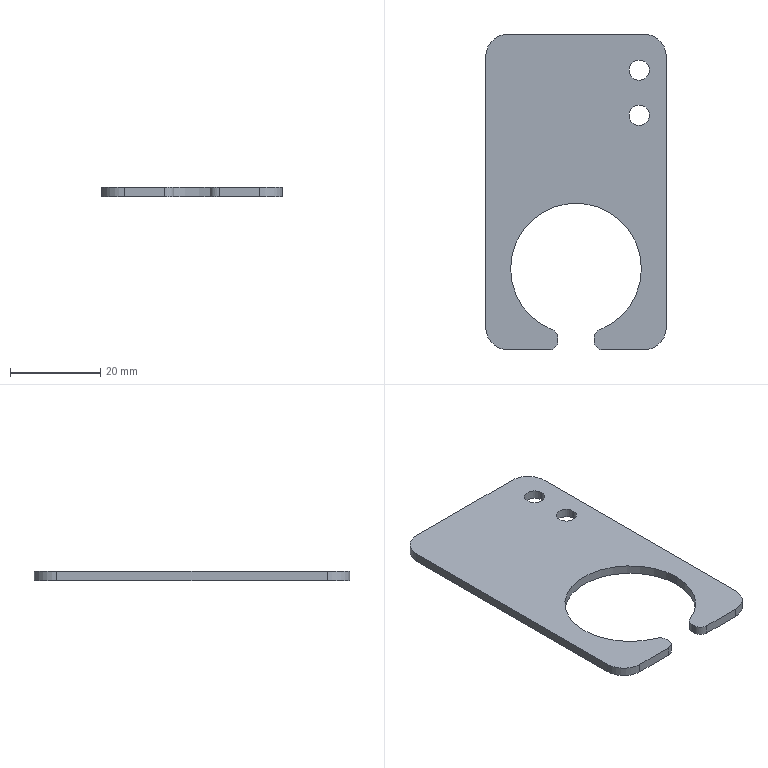Part | STEP file | 02-04 corrugated tube mounting seat (Default) | 1 solid | 24 faces | box 40 x 70 x 2 mm | volume 4109 mm3 | cylinder 15 | plane 9 | commonest cylinder face diameters 4 x4 4.5 x4 10 x4 29 x3
STEP:
#1=CARTESIAN_POINT('',(11.75,17.,-2.));
#2=VERTEX_POINT('',#1);
#3=CARTESIAN_POINT('',(16.25,17.,-2.));
#4=VERTEX_POINT('',#3);
#5=CARTESIAN_POINT('',(14.,17.,-2.));
#6=DIRECTION('',(0.,0.,1.));
#7=DIRECTION('',(1.,0.,0.));
#8=AXIS2_PLACEMENT_3D('',#5,#6,#7);
#9=CIRCLE('',#8,2.25);
#10=EDGE_CURVE('',#2,#4,#9,.T.);
#11=ORIENTED_EDGE('',*,*,#10,.F.);
#12=CARTESIAN_POINT('',(11.75,17.,0.));
#13=VERTEX_POINT('',#12);
#14=CARTESIAN_POINT('',(11.75,17.,-10.));
#15=DIRECTION('',(0.,0.,1.));
#16=VECTOR('',#15,1000.);
#17=LINE('',#14,#16);
#18=EDGE_CURVE('',#2,#13,#17,.T.);
#19=ORIENTED_EDGE('',*,*,#18,.T.);
#20=CARTESIAN_POINT('',(16.25,17.,0.));
#21=VERTEX_POINT('',#20);
#22=CARTESIAN_POINT('',(14.,17.,0.));
#23=DIRECTION('',(0.,0.,1.));
#24=DIRECTION('',(1.,0.,0.));
#25=AXIS2_PLACEMENT_3D('',#22,#23,#24);
#26=CIRCLE('',#25,2.25);
#27=EDGE_CURVE('',#13,#21,#26,.T.);
#28=ORIENTED_EDGE('',*,*,#27,.T.);
#29=CARTESIAN_POINT('',(16.25,17.,-10.));
#30=DIRECTION('',(0.,0.,1.));
#31=VECTOR('',#30,1000.);
#32=LINE('',#29,#31);
#33=EDGE_CURVE('',#4,#21,#32,.T.);
#34=ORIENTED_EDGE('',*,*,#33,.F.);
#35=EDGE_LOOP('',(#11,#19,#28,#34));
#36=FACE_OUTER_BOUND('',#35,.T.);
#37=CARTESIAN_POINT('',(14.,17.,-10.));
#38=DIRECTION('',(0.,0.,1.));
#39=DIRECTION('',(1.,0.,0.));
#40=AXIS2_PLACEMENT_3D('',#37,#38,#39);
#41=CYLINDRICAL_SURFACE('',#40,2.25);
#42=ADVANCED_FACE('',(#36),#41,.F.);
#43=CARTESIAN_POINT('',(11.75,27.,-2.));
#44=VERTEX_POINT('',#43);
#45=CARTESIAN_POINT('',(16.25,27.,-2.));
#46=VERTEX_POINT('',#45);
#47=CARTESIAN_POINT('',(14.,27.,-2.));
#48=DIRECTION('',(0.,0.,1.));
#49=DIRECTION('',(1.,0.,0.));
#50=AXIS2_PLACEMENT_3D('',#47,#48,#49);
#51=CIRCLE('',#50,2.25);
#52=EDGE_CURVE('',#44,#46,#51,.T.);
#53=ORIENTED_EDGE('',*,*,#52,.F.);
#54=CARTESIAN_POINT('',(11.75,27.,0.));
#55=VERTEX_POINT('',#54);
#56=CARTESIAN_POINT('',(11.75,27.,-10.));
#57=DIRECTION('',(0.,0.,1.));
#58=VECTOR('',#57,1000.);
#59=LINE('',#56,#58);
#60=EDGE_CURVE('',#44,#55,#59,.T.);
#61=ORIENTED_EDGE('',*,*,#60,.T.);
#62=CARTESIAN_POINT('',(16.25,27.,0.));
#63=VERTEX_POINT('',#62);
#64=CARTESIAN_POINT('',(14.,27.,0.));
#65=DIRECTION('',(0.,0.,1.));
#66=DIRECTION('',(1.,0.,0.));
#67=AXIS2_PLACEMENT_3D('',#64,#65,#66);
#68=CIRCLE('',#67,2.25);
#69=EDGE_CURVE('',#55,#63,#68,.T.);
#70=ORIENTED_EDGE('',*,*,#69,.T.);
#71=CARTESIAN_POINT('',(16.25,27.,-10.));
#72=DIRECTION('',(0.,0.,1.));
#73=VECTOR('',#72,1000.);
#74=LINE('',#71,#73);
#75=EDGE_CURVE('',#46,#63,#74,.T.);
#76=ORIENTED_EDGE('',*,*,#75,.F.);
#77=EDGE_LOOP('',(#53,#61,#70,#76));
#78=FACE_OUTER_BOUND('',#77,.T.);
#79=CARTESIAN_POINT('',(14.,27.,-10.));
#80=DIRECTION('',(0.,0.,1.));
#81=DIRECTION('',(1.,0.,0.));
#82=AXIS2_PLACEMENT_3D('',#79,#80,#81);
#83=CYLINDRICAL_SURFACE('',#82,2.25);
#84=ADVANCED_FACE('',(#78),#83,.F.);
#85=CARTESIAN_POINT('',(-14.5,-17.,-2.));
#86=VERTEX_POINT('',#85);
#87=CARTESIAN_POINT('',(-5.273,-30.507,-2.));
#88=VERTEX_POINT('',#87);
#89=CARTESIAN_POINT('',(0.,-17.,-2.));
#90=DIRECTION('',(0.,0.,1.));
#91=DIRECTION('',(1.,0.,0.));
#92=AXIS2_PLACEMENT_3D('',#89,#90,#91);
#93=CIRCLE('',#92,14.5);
#94=EDGE_CURVE('',#86,#88,#93,.T.);
#95=ORIENTED_EDGE('',*,*,#94,.F.);
#96=CARTESIAN_POINT('',(-14.5,-17.,0.));
#97=VERTEX_POINT('',#96);
#98=CARTESIAN_POINT('',(-14.5,-17.,-10.));
#99=DIRECTION('',(0.,0.,1.));
#100=VECTOR('',#99,1000.);
#101=LINE('',#98,#100);
#102=EDGE_CURVE('',#86,#97,#101,.T.);
#103=ORIENTED_EDGE('',*,*,#102,.T.);
#104=CARTESIAN_POINT('',(-5.273,-30.507,0.));
#105=VERTEX_POINT('',#104);
#106=CARTESIAN_POINT('',(0.,-17.,0.));
#107=DIRECTION('',(0.,0.,1.));
#108=DIRECTION('',(1.,0.,0.));
#109=AXIS2_PLACEMENT_3D('',#106,#107,#108);
#110=CIRCLE('',#109,14.5);
#111=EDGE_CURVE('',#97,#105,#110,.T.);
#112=ORIENTED_EDGE('',*,*,#111,.T.);
#113=CARTESIAN_POINT('',(-5.273,-30.507,-10.));
#114=DIRECTION('',(0.,0.,-1.));
#115=VECTOR('',#114,1000.);
#116=LINE('',#113,#115);
#117=EDGE_CURVE('',#105,#88,#116,.T.);
#118=ORIENTED_EDGE('',*,*,#117,.T.);
#119=EDGE_LOOP('',(#95,#103,#112,#118));
#120=FACE_OUTER_BOUND('',#119,.T.);
#121=CARTESIAN_POINT('',(0.,-17.,-10.));
#122=DIRECTION('',(0.,0.,1.));
#123=DIRECTION('',(1.,0.,0.));
#124=AXIS2_PLACEMENT_3D('',#121,#122,#123);
#125=CYLINDRICAL_SURFACE('',#124,14.5);
#126=ADVANCED_FACE('',(#120),#125,.F.);
#127=ORIENTED_EDGE('',*,*,#102,.F.);
#128=CARTESIAN_POINT('',(14.5,-17.,-2.));
#129=VERTEX_POINT('',#128);
#130=CARTESIAN_POINT('',(0.,-17.,-2.));
#131=DIRECTION('',(0.,0.,1.));
#132=DIRECTION('',(1.,0.,0.));
#133=AXIS2_PLACEMENT_3D('',#130,#131,#132);
#134=CIRCLE('',#133,14.5);
#135=EDGE_CURVE('',#129,#86,#134,.T.);
#136=ORIENTED_EDGE('',*,*,#135,.F.);
#137=CARTESIAN_POINT('',(14.5,-17.,0.));
#138=VERTEX_POINT('',#137);
#139=CARTESIAN_POINT('',(14.5,-17.,-10.));
#140=DIRECTION('',(0.,0.,1.));
#141=VECTOR('',#140,1000.);
#142=LINE('',#139,#141);
#143=EDGE_CURVE('',#129,#138,#142,.T.);
#144=ORIENTED_EDGE('',*,*,#143,.T.);
#145=CARTESIAN_POINT('',(0.,-17.,0.));
#146=DIRECTION('',(0.,0.,1.));
#147=DIRECTION('',(1.,0.,0.));
#148=AXIS2_PLACEMENT_3D('',#145,#146,#147);
#149=CIRCLE('',#148,14.5);
#150=EDGE_CURVE('',#138,#97,#149,.T.);
#151=ORIENTED_EDGE('',*,*,#150,.T.);
#152=EDGE_LOOP('',(#127,#136,#144,#151));
#153=FACE_OUTER_BOUND('',#152,.T.);
#154=CARTESIAN_POINT('',(0.,-17.,-10.));
#155=DIRECTION('',(0.,0.,1.));
#156=DIRECTION('',(1.,0.,0.));
#157=AXIS2_PLACEMENT_3D('',#154,#155,#156);
#158=CYLINDRICAL_SURFACE('',#157,14.5);
#159=ADVANCED_FACE('',(#153),#158,.F.);
#160=CARTESIAN_POINT('',(6.,-35.,-2.));
#161=VERTEX_POINT('',#160);
#162=CARTESIAN_POINT('',(15.,-35.,-2.));
#163=VERTEX_POINT('',#162);
#164=CARTESIAN_POINT('',(-20.,-35.,-2.));
#165=DIRECTION('',(1.,0.,0.));
#166=VECTOR('',#165,1000.);
#167=LINE('',#164,#166);
#168=EDGE_CURVE('',#161,#163,#167,.T.);
#169=ORIENTED_EDGE('',*,*,#168,.T.);
#170=CARTESIAN_POINT('',(15.,-35.,0.));
#171=VERTEX_POINT('',#170);
#172=CARTESIAN_POINT('',(15.,-35.,-2.));
#173=DIRECTION('',(0.,0.,1.));
#174=VECTOR('',#173,1000.);
#175=LINE('',#172,#174);
#176=EDGE_CURVE('',#163,#171,#175,.T.);
#177=ORIENTED_EDGE('',*,*,#176,.T.);
#178=CARTESIAN_POINT('',(6.,-35.,0.));
#179=VERTEX_POINT('',#178);
#180=CARTESIAN_POINT('',(-20.,-35.,0.));
#181=DIRECTION('',(1.,0.,0.));
#182=VECTOR('',#181,1000.);
#183=LINE('',#180,#182);
#184=EDGE_CURVE('',#179,#171,#183,.T.);
#185=ORIENTED_EDGE('',*,*,#184,.F.);
#186=CARTESIAN_POINT('',(6.,-35.,-2.));
#187=DIRECTION('',(0.,0.,-1.));
#188=VECTOR('',#187,1000.);
#189=LINE('',#186,#188);
#190=EDGE_CURVE('',#179,#161,#189,.T.);
#191=ORIENTED_EDGE('',*,*,#190,.T.);
#192=EDGE_LOOP('',(#169,#177,#185,#191));
#193=FACE_OUTER_BOUND('',#192,.T.);
#194=CARTESIAN_POINT('',(-20.,-35.,-2.));
#195=DIRECTION('',(0.,-1.,0.));
#196=DIRECTION('',(0.,0.,-1.));
#197=AXIS2_PLACEMENT_3D('',#194,#195,#196);
#198=PLANE('',#197);
#199=ADVANCED_FACE('',(#193),#198,.T.);
#200=CARTESIAN_POINT('',(20.,-30.,-2.));
#201=VERTEX_POINT('',#200);
#202=CARTESIAN_POINT('',(20.,30.,-2.));
#203=VERTEX_POINT('',#202);
#204=CARTESIAN_POINT('',(20.,35.,-2.));
#205=DIRECTION('',(0.,1.,0.));
#206=VECTOR('',#205,1000.);
#207=LINE('',#204,#206);
#208=EDGE_CURVE('',#201,#203,#207,.T.);
#209=ORIENTED_EDGE('',*,*,#208,.T.);
#210=CARTESIAN_POINT('',(20.,30.,0.));
#211=VERTEX_POINT('',#210);
#212=CARTESIAN_POINT('',(20.,30.,-2.));
#213=DIRECTION('',(0.,0.,1.));
#214=VECTOR('',#213,1000.);
#215=LINE('',#212,#214);
#216=EDGE_CURVE('',#203,#211,#215,.T.);
#217=ORIENTED_EDGE('',*,*,#216,.T.);
#218=CARTESIAN_POINT('',(20.,-30.,0.));
#219=VERTEX_POINT('',#218);
#220=CARTESIAN_POINT('',(20.,35.,0.));
#221=DIRECTION('',(0.,1.,0.));
#222=VECTOR('',#221,1000.);
#223=LINE('',#220,#222);
#224=EDGE_CURVE('',#219,#211,#223,.T.);
#225=ORIENTED_EDGE('',*,*,#224,.F.);
#226=CARTESIAN_POINT('',(20.,-30.,-2.));
#227=DIRECTION('',(0.,0.,-1.));
#228=VECTOR('',#227,1000.);
#229=LINE('',#226,#228);
#230=EDGE_CURVE('',#219,#201,#229,.T.);
#231=ORIENTED_EDGE('',*,*,#230,.T.);
#232=EDGE_LOOP('',(#209,#217,#225,#231));
#233=FACE_OUTER_BOUND('',#232,.T.);
#234=CARTESIAN_POINT('',(20.,35.,-2.));
#235=DIRECTION('',(1.,0.,0.));
#236=DIRECTION('',(0.,1.,0.));
#237=AXIS2_PLACEMENT_3D('',#234,#235,#236);
#238=PLANE('',#237);
#239=ADVANCED_FACE('',(#233),#238,.T.);
#240=CARTESIAN_POINT('',(-15.,-35.,0.));
#241=VERTEX_POINT('',#240);
#242=CARTESIAN_POINT('',(-6.,-35.,0.));
#243=VERTEX_POINT('',#242);
#244=CARTESIAN_POINT('',(-20.,-35.,0.));
#245=DIRECTION('',(1.,0.,0.));
#246=VECTOR('',#245,1000.);
#247=LINE('',#244,#246);
#248=EDGE_CURVE('',#241,#243,#247,.T.);
#249=ORIENTED_EDGE('',*,*,#248,.F.);
#250=CARTESIAN_POINT('',(-15.,-35.,-2.));
#251=VERTEX_POINT('',#250);
#252=CARTESIAN_POINT('',(-15.,-35.,-2.));
#253=DIRECTION('',(0.,0.,-1.));
#254=VECTOR('',#253,1000.);
#255=LINE('',#252,#254);
#256=EDGE_CURVE('',#241,#251,#255,.T.);
#257=ORIENTED_EDGE('',*,*,#256,.T.);
#258=CARTESIAN_POINT('',(-6.,-35.,-2.));
#259=VERTEX_POINT('',#258);
#260=CARTESIAN_POINT('',(-20.,-35.,-2.));
#261=DIRECTION('',(1.,0.,0.));
#262=VECTOR('',#261,1000.);
#263=LINE('',#260,#262);
#264=EDGE_CURVE('',#251,#259,#263,.T.);
#265=ORIENTED_EDGE('',*,*,#264,.T.);
#266=CARTESIAN_POINT('',(-6.,-35.,0.));
#267=DIRECTION('',(0.,0.,1.));
#268=VECTOR('',#267,1000.);
#269=LINE('',#266,#268);
#270=EDGE_CURVE('',#259,#243,#269,.T.);
#271=ORIENTED_EDGE('',*,*,#270,.T.);
#272=EDGE_LOOP('',(#249,#257,#265,#271));
#273=FACE_OUTER_BOUND('',#272,.T.);
#274=CARTESIAN_POINT('',(-20.,-35.,-2.));
#275=DIRECTION('',(0.,-1.,0.));
#276=DIRECTION('',(0.,0.,-1.));
#277=AXIS2_PLACEMENT_3D('',#274,#275,#276);
#278=PLANE('',#277);
#279=ADVANCED_FACE('',(#273),#278,.T.);
#280=CARTESIAN_POINT('',(-20.,30.,0.));
#281=VERTEX_POINT('',#280);
#282=CARTESIAN_POINT('',(-20.,-30.,0.));
#283=VERTEX_POINT('',#282);
#284=CARTESIAN_POINT('',(-20.,35.,0.));
#285=DIRECTION('',(0.,-1.,0.));
#286=VECTOR('',#285,1000.);
#287=LINE('',#284,#286);
#288=EDGE_CURVE('',#281,#283,#287,.T.);
#289=ORIENTED_EDGE('',*,*,#288,.F.);
#290=CARTESIAN_POINT('',(-20.,30.,-2.));
#291=VERTEX_POINT('',#290);
#292=CARTESIAN_POINT('',(-20.,30.,-2.));
#293=DIRECTION('',(0.,0.,-1.));
#294=VECTOR('',#293,1000.);
#295=LINE('',#292,#294);
#296=EDGE_CURVE('',#281,#291,#295,.T.);
#297=ORIENTED_EDGE('',*,*,#296,.T.);
#298=CARTESIAN_POINT('',(-20.,-30.,-2.));
#299=VERTEX_POINT('',#298);
#300=CARTESIAN_POINT('',(-20.,35.,-2.));
#301=DIRECTION('',(0.,-1.,0.));
#302=VECTOR('',#301,1000.);
#303=LINE('',#300,#302);
#304=EDGE_CURVE('',#291,#299,#303,.T.);
#305=ORIENTED_EDGE('',*,*,#304,.T.);
#306=CARTESIAN_POINT('',(-20.,-30.,-2.));
#307=DIRECTION('',(0.,0.,1.));
#308=VECTOR('',#307,1000.);
#309=LINE('',#306,#308);
#310=EDGE_CURVE('',#299,#283,#309,.T.);
#311=ORIENTED_EDGE('',*,*,#310,.T.);
#312=EDGE_LOOP('',(#289,#297,#305,#311));
#313=FACE_OUTER_BOUND('',#312,.T.);
#314=CARTESIAN_POINT('',(-20.,35.,-2.));
#315=DIRECTION('',(-1.,0.,0.));
#316=DIRECTION('',(0.,-1.,0.));
#317=AXIS2_PLACEMENT_3D('',#314,#315,#316);
#318=PLANE('',#317);
#319=ADVANCED_FACE('',(#313),#318,.T.);
#320=CARTESIAN_POINT('',(15.,35.,0.));
#321=VERTEX_POINT('',#320);
#322=CARTESIAN_POINT('',(-15.,35.,0.));
#323=VERTEX_POINT('',#322);
#324=CARTESIAN_POINT('',(-20.,35.,0.));
#325=DIRECTION('',(-1.,0.,0.));
#326=VECTOR('',#325,1000.);
#327=LINE('',#324,#326);
#328=EDGE_CURVE('',#321,#323,#327,.T.);
#329=ORIENTED_EDGE('',*,*,#328,.F.);
#330=CARTESIAN_POINT('',(15.,35.,-2.));
#331=VERTEX_POINT('',#330);
#332=CARTESIAN_POINT('',(15.,35.,-2.));
#333=DIRECTION('',(0.,0.,-1.));
#334=VECTOR('',#333,1000.);
#335=LINE('',#332,#334);
#336=EDGE_CURVE('',#321,#331,#335,.T.);
#337=ORIENTED_EDGE('',*,*,#336,.T.);
#338=CARTESIAN_POINT('',(-15.,35.,-2.));
#339=VERTEX_POINT('',#338);
#340=CARTESIAN_POINT('',(-20.,35.,-2.));
#341=DIRECTION('',(-1.,0.,0.));
#342=VECTOR('',#341,1000.);
#343=LINE('',#340,#342);
#344=EDGE_CURVE('',#331,#339,#343,.T.);
#345=ORIENTED_EDGE('',*,*,#344,.T.);
#346=CARTESIAN_POINT('',(-15.,35.,-2.));
#347=DIRECTION('',(0.,0.,1.));
#348=VECTOR('',#347,1000.);
#349=LINE('',#346,#348);
#350=EDGE_CURVE('',#339,#323,#349,.T.);
#351=ORIENTED_EDGE('',*,*,#350,.T.);
#352=EDGE_LOOP('',(#329,#337,#345,#351));
#353=FACE_OUTER_BOUND('',#352,.T.);
#354=CARTESIAN_POINT('',(-20.,35.,-2.));
#355=DIRECTION('',(0.,1.,0.));
#356=DIRECTION('',(0.,0.,1.));
#357=AXIS2_PLACEMENT_3D('',#354,#355,#356);
#358=PLANE('',#357);
#359=ADVANCED_FACE('',(#353),#358,.T.);
#360=CARTESIAN_POINT('',(14.,17.,-2.));
#361=DIRECTION('',(0.,0.,1.));
#362=DIRECTION('',(1.,0.,0.));
#363=AXIS2_PLACEMENT_3D('',#360,#361,#362);
#364=CIRCLE('',#363,2.25);
#365=EDGE_CURVE('',#4,#2,#364,.T.);
#366=ORIENTED_EDGE('',*,*,#365,.T.);
#367=ORIENTED_EDGE('',*,*,#10,.T.);
#368=EDGE_LOOP('',(#366,#367));
#369=FACE_BOUND('',#368,.T.);
#370=CARTESIAN_POINT('',(14.,27.,-2.));
#371=DIRECTION('',(0.,0.,1.));
#372=DIRECTION('',(1.,0.,0.));
#373=AXIS2_PLACEMENT_3D('',#370,#371,#372);
#374=CIRCLE('',#373,2.25);
#375=EDGE_CURVE('',#46,#44,#374,.T.);
#376=ORIENTED_EDGE('',*,*,#375,.T.);
#377=ORIENTED_EDGE('',*,*,#52,.T.);
#378=EDGE_LOOP('',(#376,#377));
#379=FACE_BOUND('',#378,.T.);
#380=ORIENTED_EDGE('',*,*,#344,.F.);
#381=CARTESIAN_POINT('',(15.,30.,-2.));
#382=DIRECTION('',(0.,0.,-1.));
#383=DIRECTION('',(1.,0.,0.));
#384=AXIS2_PLACEMENT_3D('',#381,#382,#383);
#385=CIRCLE('',#384,5.);
#386=EDGE_CURVE('',#331,#203,#385,.T.);
#387=ORIENTED_EDGE('',*,*,#386,.T.);
#388=ORIENTED_EDGE('',*,*,#208,.F.);
#389=CARTESIAN_POINT('',(15.,-30.,-2.));
#390=DIRECTION('',(0.,0.,-1.));
#391=DIRECTION('',(1.,0.,0.));
#392=AXIS2_PLACEMENT_3D('',#389,#390,#391);
#393=CIRCLE('',#392,5.);
#394=EDGE_CURVE('',#201,#163,#393,.T.);
#395=ORIENTED_EDGE('',*,*,#394,.T.);
#396=ORIENTED_EDGE('',*,*,#168,.F.);
#397=CARTESIAN_POINT('',(4.,-33.,-2.));
#398=VERTEX_POINT('',#397);
#399=CARTESIAN_POINT('',(6.,-33.,-2.));
#400=DIRECTION('',(0.,0.,-1.));
#401=DIRECTION('',(1.,0.,0.));
#402=AXIS2_PLACEMENT_3D('',#399,#400,#401);
#403=CIRCLE('',#402,2.);
#404=EDGE_CURVE('',#161,#398,#403,.T.);
#405=ORIENTED_EDGE('',*,*,#404,.T.);
#406=CARTESIAN_POINT('',(4.,-32.37,-2.));
#407=VERTEX_POINT('',#406);
#408=CARTESIAN_POINT('',(4.,-35.,-2.));
#409=DIRECTION('',(0.,1.,0.));
#410=VECTOR('',#409,1000.);
#411=LINE('',#408,#410);
#412=EDGE_CURVE('',#398,#407,#411,.T.);
#413=ORIENTED_EDGE('',*,*,#412,.T.);
#414=CARTESIAN_POINT('',(5.273,-30.507,-2.));
#415=VERTEX_POINT('',#414);
#416=CARTESIAN_POINT('',(6.,-32.37,-2.));
#417=DIRECTION('',(0.,0.,-1.));
#418=DIRECTION('',(1.,0.,0.));
#419=AXIS2_PLACEMENT_3D('',#416,#417,#418);
#420=CIRCLE('',#419,2.);
#421=EDGE_CURVE('',#407,#415,#420,.T.);
#422=ORIENTED_EDGE('',*,*,#421,.T.);
#423=CARTESIAN_POINT('',(0.,-17.,-2.));
#424=DIRECTION('',(0.,0.,1.));
#425=DIRECTION('',(1.,0.,0.));
#426=AXIS2_PLACEMENT_3D('',#423,#424,#425);
#427=CIRCLE('',#426,14.5);
#428=EDGE_CURVE('',#415,#129,#427,.T.);
#429=ORIENTED_EDGE('',*,*,#428,.T.);
#430=ORIENTED_EDGE('',*,*,#135,.T.);
#431=ORIENTED_EDGE('',*,*,#94,.T.);
#432=CARTESIAN_POINT('',(-4.,-32.37,-2.));
#433=VERTEX_POINT('',#432);
#434=CARTESIAN_POINT('',(-6.,-32.37,-2.));
#435=DIRECTION('',(0.,0.,-1.));
#436=DIRECTION('',(1.,0.,0.));
#437=AXIS2_PLACEMENT_3D('',#434,#435,#436);
#438=CIRCLE('',#437,2.);
#439=EDGE_CURVE('',#88,#433,#438,.T.);
#440=ORIENTED_EDGE('',*,*,#439,.T.);
#441=CARTESIAN_POINT('',(-4.,-33.,-2.));
#442=VERTEX_POINT('',#441);
#443=CARTESIAN_POINT('',(-4.,-35.,-2.));
#444=DIRECTION('',(0.,-1.,0.));
#445=VECTOR('',#444,1000.);
#446=LINE('',#443,#445);
#447=EDGE_CURVE('',#433,#442,#446,.T.);
#448=ORIENTED_EDGE('',*,*,#447,.T.);
#449=CARTESIAN_POINT('',(-6.,-33.,-2.));
#450=DIRECTION('',(0.,0.,-1.));
#451=DIRECTION('',(1.,0.,0.));
#452=AXIS2_PLACEMENT_3D('',#449,#450,#451);
#453=CIRCLE('',#452,2.);
#454=EDGE_CURVE('',#442,#259,#453,.T.);
#455=ORIENTED_EDGE('',*,*,#454,.T.);
#456=ORIENTED_EDGE('',*,*,#264,.F.);
#457=CARTESIAN_POINT('',(-15.,-30.,-2.));
#458=DIRECTION('',(0.,0.,-1.));
#459=DIRECTION('',(1.,0.,0.));
#460=AXIS2_PLACEMENT_3D('',#457,#458,#459);
#461=CIRCLE('',#460,5.);
#462=EDGE_CURVE('',#251,#299,#461,.T.);
#463=ORIENTED_EDGE('',*,*,#462,.T.);
#464=ORIENTED_EDGE('',*,*,#304,.F.);
#465=CARTESIAN_POINT('',(-15.,30.,-2.));
#466=DIRECTION('',(0.,0.,-1.));
#467=DIRECTION('',(1.,0.,0.));
#468=AXIS2_PLACEMENT_3D('',#465,#466,#467);
#469=CIRCLE('',#468,5.);
#470=EDGE_CURVE('',#291,#339,#469,.T.);
#471=ORIENTED_EDGE('',*,*,#470,.T.);
#472=EDGE_LOOP('',(#380,#387,#388,#395,#396,#405,#413,#422,#429,#430,#431,#440,#448,#455,#456,#463,#464,#471));
#473=FACE_OUTER_BOUND('',#472,.T.);
#474=CARTESIAN_POINT('',(20.,-35.,-2.));
#475=DIRECTION('',(0.,0.,1.));
#476=DIRECTION('',(1.,0.,0.));
#477=AXIS2_PLACEMENT_3D('',#474,#475,#476);
#478=PLANE('',#477);
#479=ADVANCED_FACE('',(#369,#379,#473),#478,.F.);
#480=CARTESIAN_POINT('',(14.,17.,0.));
#481=DIRECTION('',(0.,0.,1.));
#482=DIRECTION('',(1.,0.,0.));
#483=AXIS2_PLACEMENT_3D('',#480,#481,#482);
#484=CIRCLE('',#483,2.25);
#485=EDGE_CURVE('',#21,#13,#484,.T.);
#486=ORIENTED_EDGE('',*,*,#485,.F.);
#487=ORIENTED_EDGE('',*,*,#27,.F.);
#488=EDGE_LOOP('',(#486,#487));
#489=FACE_BOUND('',#488,.T.);
#490=CARTESIAN_POINT('',(14.,27.,0.));
#491=DIRECTION('',(0.,0.,1.));
#492=DIRECTION('',(1.,0.,0.));
#493=AXIS2_PLACEMENT_3D('',#490,#491,#492);
#494=CIRCLE('',#493,2.25);
#495=EDGE_CURVE('',#63,#55,#494,.T.);
#496=ORIENTED_EDGE('',*,*,#495,.F.);
#497=ORIENTED_EDGE('',*,*,#69,.F.);
#498=EDGE_LOOP('',(#496,#497));
#499=FACE_BOUND('',#498,.T.);
#500=ORIENTED_EDGE('',*,*,#224,.T.);
#501=CARTESIAN_POINT('',(15.,30.,0.));
#502=DIRECTION('',(0.,0.,1.));
#503=DIRECTION('',(1.,0.,0.));
#504=AXIS2_PLACEMENT_3D('',#501,#502,#503);
#505=CIRCLE('',#504,5.);
#506=EDGE_CURVE('',#211,#321,#505,.T.);
#507=ORIENTED_EDGE('',*,*,#506,.T.);
#508=ORIENTED_EDGE('',*,*,#328,.T.);
#509=CARTESIAN_POINT('',(-15.,30.,0.));
#510=DIRECTION('',(0.,0.,1.));
#511=DIRECTION('',(1.,0.,0.));
#512=AXIS2_PLACEMENT_3D('',#509,#510,#511);
#513=CIRCLE('',#512,5.);
#514=EDGE_CURVE('',#323,#281,#513,.T.);
#515=ORIENTED_EDGE('',*,*,#514,.T.);
#516=ORIENTED_EDGE('',*,*,#288,.T.);
#517=CARTESIAN_POINT('',(-15.,-30.,0.));
#518=DIRECTION('',(0.,0.,1.));
#519=DIRECTION('',(1.,0.,0.));
#520=AXIS2_PLACEMENT_3D('',#517,#518,#519);
#521=CIRCLE('',#520,5.);
#522=EDGE_CURVE('',#283,#241,#521,.T.);
#523=ORIENTED_EDGE('',*,*,#522,.T.);
#524=ORIENTED_EDGE('',*,*,#248,.T.);
#525=CARTESIAN_POINT('',(-4.,-33.,0.));
#526=VERTEX_POINT('',#525);
#527=CARTESIAN_POINT('',(-6.,-33.,0.));
#528=DIRECTION('',(0.,0.,1.));
#529=DIRECTION('',(1.,0.,0.));
#530=AXIS2_PLACEMENT_3D('',#527,#528,#529);
#531=CIRCLE('',#530,2.);
#532=EDGE_CURVE('',#243,#526,#531,.T.);
#533=ORIENTED_EDGE('',*,*,#532,.T.);
#534=CARTESIAN_POINT('',(-4.,-32.37,0.));
#535=VERTEX_POINT('',#534);
#536=CARTESIAN_POINT('',(-4.,-30.937,0.));
#537=DIRECTION('',(0.,-1.,0.));
#538=VECTOR('',#537,1000.);
#539=LINE('',#536,#538);
#540=EDGE_CURVE('',#535,#526,#539,.T.);
#541=ORIENTED_EDGE('',*,*,#540,.F.);
#542=CARTESIAN_POINT('',(-6.,-32.37,0.));
#543=DIRECTION('',(0.,0.,1.));
#544=DIRECTION('',(1.,0.,0.));
#545=AXIS2_PLACEMENT_3D('',#542,#543,#544);
#546=CIRCLE('',#545,2.);
#547=EDGE_CURVE('',#535,#105,#546,.T.);
#548=ORIENTED_EDGE('',*,*,#547,.T.);
#549=ORIENTED_EDGE('',*,*,#111,.F.);
#550=ORIENTED_EDGE('',*,*,#150,.F.);
#551=CARTESIAN_POINT('',(5.273,-30.507,0.));
#552=VERTEX_POINT('',#551);
#553=CARTESIAN_POINT('',(0.,-17.,0.));
#554=DIRECTION('',(0.,0.,1.));
#555=DIRECTION('',(1.,0.,0.));
#556=AXIS2_PLACEMENT_3D('',#553,#554,#555);
#557=CIRCLE('',#556,14.5);
#558=EDGE_CURVE('',#552,#138,#557,.T.);
#559=ORIENTED_EDGE('',*,*,#558,.F.);
#560=CARTESIAN_POINT('',(4.,-32.37,0.));
#561=VERTEX_POINT('',#560);
#562=CARTESIAN_POINT('',(6.,-32.37,0.));
#563=DIRECTION('',(0.,0.,1.));
#564=DIRECTION('',(1.,0.,0.));
#565=AXIS2_PLACEMENT_3D('',#562,#563,#564);
#566=CIRCLE('',#565,2.);
#567=EDGE_CURVE('',#552,#561,#566,.T.);
#568=ORIENTED_EDGE('',*,*,#567,.T.);
#569=CARTESIAN_POINT('',(4.,-33.,0.));
#570=VERTEX_POINT('',#569);
#571=CARTESIAN_POINT('',(4.,-35.,0.));
#572=DIRECTION('',(0.,1.,0.));
#573=VECTOR('',#572,1000.);
#574=LINE('',#571,#573);
#575=EDGE_CURVE('',#570,#561,#574,.T.);
#576=ORIENTED_EDGE('',*,*,#575,.F.);
#577=CARTESIAN_POINT('',(6.,-33.,0.));
#578=DIRECTION('',(0.,0.,1.));
#579=DIRECTION('',(1.,0.,0.));
#580=AXIS2_PLACEMENT_3D('',#577,#578,#579);
#581=CIRCLE('',#580,2.);
#582=EDGE_CURVE('',#570,#179,#581,.T.);
#583=ORIENTED_EDGE('',*,*,#582,.T.);
#584=ORIENTED_EDGE('',*,*,#184,.T.);
#585=CARTESIAN_POINT('',(15.,-30.,0.));
#586=DIRECTION('',(0.,0.,1.));
#587=DIRECTION('',(1.,0.,0.));
#588=AXIS2_PLACEMENT_3D('',#585,#586,#587);
#589=CIRCLE('',#588,5.);
#590=EDGE_CURVE('',#171,#219,#589,.T.);
#591=ORIENTED_EDGE('',*,*,#590,.T.);
#592=EDGE_LOOP('',(#500,#507,#508,#515,#516,#523,#524,#533,#541,#548,#549,#550,#559,#568,#576,#583,#584,#591));
#593=FACE_OUTER_BOUND('',#592,.T.);
#594=CARTESIAN_POINT('',(20.,-35.,0.));
#595=DIRECTION('',(0.,0.,1.));
#596=DIRECTION('',(1.,0.,0.));
#597=AXIS2_PLACEMENT_3D('',#594,#595,#596);
#598=PLANE('',#597);
#599=ADVANCED_FACE('',(#489,#499,#593),#598,.T.);
#600=ORIENTED_EDGE('',*,*,#143,.F.);
#601=ORIENTED_EDGE('',*,*,#428,.F.);
#602=CARTESIAN_POINT('',(5.273,-30.507,-10.));
#603=DIRECTION('',(0.,0.,1.));
#604=VECTOR('',#603,1000.);
#605=LINE('',#602,#604);
#606=EDGE_CURVE('',#415,#552,#605,.T.);
#607=ORIENTED_EDGE('',*,*,#606,.T.);
#608=ORIENTED_EDGE('',*,*,#558,.T.);
#609=EDGE_LOOP('',(#600,#601,#607,#608));
#610=FACE_OUTER_BOUND('',#609,.T.);
#611=CARTESIAN_POINT('',(0.,-17.,-10.));
#612=DIRECTION('',(0.,0.,1.));
#613=DIRECTION('',(1.,0.,0.));
#614=AXIS2_PLACEMENT_3D('',#611,#612,#613);
#615=CYLINDRICAL_SURFACE('',#614,14.5);
#616=ADVANCED_FACE('',(#610),#615,.F.);
#617=ORIENTED_EDGE('',*,*,#412,.F.);
#618=CARTESIAN_POINT('',(4.,-33.,0.));
#619=DIRECTION('',(0.,0.,1.));
#620=VECTOR('',#619,1000.);
#621=LINE('',#618,#620);
#622=EDGE_CURVE('',#398,#570,#621,.T.);
#623=ORIENTED_EDGE('',*,*,#622,.T.);
#624=ORIENTED_EDGE('',*,*,#575,.T.);
#625=CARTESIAN_POINT('',(4.,-32.37,-10.));
#626=DIRECTION('',(0.,0.,-1.));
#627=VECTOR('',#626,1000.);
#628=LINE('',#625,#627);
#629=EDGE_CURVE('',#561,#407,#628,.T.);
#630=ORIENTED_EDGE('',*,*,#629,.T.);
#631=EDGE_LOOP('',(#617,#623,#624,#630));
#632=FACE_OUTER_BOUND('',#631,.T.);
#633=CARTESIAN_POINT('',(4.,-30.937,-10.));
#634=DIRECTION('',(1.,0.,0.));
#635=DIRECTION('',(0.,0.,-1.));
#636=AXIS2_PLACEMENT_3D('',#633,#634,#635);
#637=PLANE('',#636);
#638=ADVANCED_FACE('',(#632),#637,.F.);
#639=ORIENTED_EDGE('',*,*,#540,.T.);
#640=CARTESIAN_POINT('',(-4.,-33.,-2.));
#641=DIRECTION('',(0.,0.,-1.));
#642=VECTOR('',#641,1000.);
#643=LINE('',#640,#642);
#644=EDGE_CURVE('',#526,#442,#643,.T.);
#645=ORIENTED_EDGE('',*,*,#644,.T.);
#646=ORIENTED_EDGE('',*,*,#447,.F.);
#647=CARTESIAN_POINT('',(-4.,-32.37,-10.));
#648=DIRECTION('',(0.,0.,1.));
#649=VECTOR('',#648,1000.);
#650=LINE('',#647,#649);
#651=EDGE_CURVE('',#433,#535,#650,.T.);
#652=ORIENTED_EDGE('',*,*,#651,.T.);
#653=EDGE_LOOP('',(#639,#645,#646,#652));
#654=FACE_OUTER_BOUND('',#653,.T.);
#655=CARTESIAN_POINT('',(-4.,-30.937,-10.));
#656=DIRECTION('',(-1.,0.,0.));
#657=DIRECTION('',(0.,0.,1.));
#658=AXIS2_PLACEMENT_3D('',#655,#656,#657);
#659=PLANE('',#658);
#660=ADVANCED_FACE('',(#654),#659,.F.);
#661=ORIENTED_EDGE('',*,*,#404,.F.);
#662=ORIENTED_EDGE('',*,*,#190,.F.);
#663=ORIENTED_EDGE('',*,*,#582,.F.);
#664=ORIENTED_EDGE('',*,*,#622,.F.);
#665=EDGE_LOOP('',(#661,#662,#663,#664));
#666=FACE_OUTER_BOUND('',#665,.T.);
#667=CARTESIAN_POINT('',(6.,-33.,-10.));
#668=DIRECTION('',(0.,0.,-1.));
#669=DIRECTION('',(-1.,0.,0.));
#670=AXIS2_PLACEMENT_3D('',#667,#668,#669);
#671=CYLINDRICAL_SURFACE('',#670,2.);
#672=ADVANCED_FACE('',(#666),#671,.T.);
#673=ORIENTED_EDGE('',*,*,#532,.F.);
#674=ORIENTED_EDGE('',*,*,#270,.F.);
#675=ORIENTED_EDGE('',*,*,#454,.F.);
#676=ORIENTED_EDGE('',*,*,#644,.F.);
#677=EDGE_LOOP('',(#673,#674,#675,#676));
#678=FACE_OUTER_BOUND('',#677,.T.);
#679=CARTESIAN_POINT('',(-6.,-33.,-10.));
#680=DIRECTION('',(0.,0.,1.));
#681=DIRECTION('',(1.,0.,0.));
#682=AXIS2_PLACEMENT_3D('',#679,#680,#681);
#683=CYLINDRICAL_SURFACE('',#682,2.);
#684=ADVANCED_FACE('',(#678),#683,.T.);
#685=ORIENTED_EDGE('',*,*,#421,.F.);
#686=ORIENTED_EDGE('',*,*,#629,.F.);
#687=ORIENTED_EDGE('',*,*,#567,.F.);
#688=ORIENTED_EDGE('',*,*,#606,.F.);
#689=EDGE_LOOP('',(#685,#686,#687,#688));
#690=FACE_OUTER_BOUND('',#689,.T.);
#691=CARTESIAN_POINT('',(6.,-32.37,-10.));
#692=DIRECTION('',(0.,0.,1.));
#693=DIRECTION('',(1.,0.,0.));
#694=AXIS2_PLACEMENT_3D('',#691,#692,#693);
#695=CYLINDRICAL_SURFACE('',#694,2.);
#696=ADVANCED_FACE('',(#690),#695,.T.);
#697=ORIENTED_EDGE('',*,*,#439,.F.);
#698=ORIENTED_EDGE('',*,*,#117,.F.);
#699=ORIENTED_EDGE('',*,*,#547,.F.);
#700=ORIENTED_EDGE('',*,*,#651,.F.);
#701=EDGE_LOOP('',(#697,#698,#699,#700));
#702=FACE_OUTER_BOUND('',#701,.T.);
#703=CARTESIAN_POINT('',(-6.,-32.37,-10.));
#704=DIRECTION('',(0.,0.,1.));
#705=DIRECTION('',(1.,0.,0.));
#706=AXIS2_PLACEMENT_3D('',#703,#704,#705);
#707=CYLINDRICAL_SURFACE('',#706,2.);
#708=ADVANCED_FACE('',(#702),#707,.T.);
#709=ORIENTED_EDGE('',*,*,#386,.F.);
#710=ORIENTED_EDGE('',*,*,#336,.F.);
#711=ORIENTED_EDGE('',*,*,#506,.F.);
#712=ORIENTED_EDGE('',*,*,#216,.F.);
#713=EDGE_LOOP('',(#709,#710,#711,#712));
#714=FACE_OUTER_BOUND('',#713,.T.);
#715=CARTESIAN_POINT('',(15.,30.,-2.));
#716=DIRECTION('',(0.,0.,1.));
#717=DIRECTION('',(1.,0.,0.));
#718=AXIS2_PLACEMENT_3D('',#715,#716,#717);
#719=CYLINDRICAL_SURFACE('',#718,5.);
#720=ADVANCED_FACE('',(#714),#719,.T.);
#721=ORIENTED_EDGE('',*,*,#470,.F.);
#722=ORIENTED_EDGE('',*,*,#296,.F.);
#723=ORIENTED_EDGE('',*,*,#514,.F.);
#724=ORIENTED_EDGE('',*,*,#350,.F.);
#725=EDGE_LOOP('',(#721,#722,#723,#724));
#726=FACE_OUTER_BOUND('',#725,.T.);
#727=CARTESIAN_POINT('',(-15.,30.,-2.));
#728=DIRECTION('',(0.,0.,1.));
#729=DIRECTION('',(1.,0.,0.));
#730=AXIS2_PLACEMENT_3D('',#727,#728,#729);
#731=CYLINDRICAL_SURFACE('',#730,5.);
#732=ADVANCED_FACE('',(#726),#731,.T.);
#733=ORIENTED_EDGE('',*,*,#394,.F.);
#734=ORIENTED_EDGE('',*,*,#230,.F.);
#735=ORIENTED_EDGE('',*,*,#590,.F.);
#736=ORIENTED_EDGE('',*,*,#176,.F.);
#737=EDGE_LOOP('',(#733,#734,#735,#736));
#738=FACE_OUTER_BOUND('',#737,.T.);
#739=CARTESIAN_POINT('',(15.,-30.,-2.));
#740=DIRECTION('',(0.,0.,1.));
#741=DIRECTION('',(1.,0.,0.));
#742=AXIS2_PLACEMENT_3D('',#739,#740,#741);
#743=CYLINDRICAL_SURFACE('',#742,5.);
#744=ADVANCED_FACE('',(#738),#743,.T.);
#745=ORIENTED_EDGE('',*,*,#462,.F.);
#746=ORIENTED_EDGE('',*,*,#256,.F.);
#747=ORIENTED_EDGE('',*,*,#522,.F.);
#748=ORIENTED_EDGE('',*,*,#310,.F.);
#749=EDGE_LOOP('',(#745,#746,#747,#748));
#750=FACE_OUTER_BOUND('',#749,.T.);
#751=CARTESIAN_POINT('',(-15.,-30.,-2.));
#752=DIRECTION('',(0.,0.,1.));
#753=DIRECTION('',(1.,0.,0.));
#754=AXIS2_PLACEMENT_3D('',#751,#752,#753);
#755=CYLINDRICAL_SURFACE('',#754,5.);
#756=ADVANCED_FACE('',(#750),#755,.T.);
#757=ORIENTED_EDGE('',*,*,#60,.F.);
#758=ORIENTED_EDGE('',*,*,#375,.F.);
#759=ORIENTED_EDGE('',*,*,#75,.T.);
#760=ORIENTED_EDGE('',*,*,#495,.T.);
#761=EDGE_LOOP('',(#757,#758,#759,#760));
#762=FACE_OUTER_BOUND('',#761,.T.);
#763=CARTESIAN_POINT('',(14.,27.,-10.));
#764=DIRECTION('',(0.,0.,1.));
#765=DIRECTION('',(1.,0.,0.));
#766=AXIS2_PLACEMENT_3D('',#763,#764,#765);
#767=CYLINDRICAL_SURFACE('',#766,2.25);
#768=ADVANCED_FACE('',(#762),#767,.F.);
#769=ORIENTED_EDGE('',*,*,#18,.F.);
#770=ORIENTED_EDGE('',*,*,#365,.F.);
#771=ORIENTED_EDGE('',*,*,#33,.T.);
#772=ORIENTED_EDGE('',*,*,#485,.T.);
#773=EDGE_LOOP('',(#769,#770,#771,#772));
#774=FACE_OUTER_BOUND('',#773,.T.);
#775=CARTESIAN_POINT('',(14.,17.,-10.));
#776=DIRECTION('',(0.,0.,1.));
#777=DIRECTION('',(1.,0.,0.));
#778=AXIS2_PLACEMENT_3D('',#775,#776,#777);
#779=CYLINDRICAL_SURFACE('',#778,2.25);
#780=ADVANCED_FACE('',(#774),#779,.F.);
#781=CLOSED_SHELL('',(#42,#84,#126,#159,#199,#239,#279,#319,#359,#479,#599,#616,#638,#660,#672,#684,#696,#708,#720,#732,#744,#756,#768,#780));
#782=MANIFOLD_SOLID_BREP('',#781);
#783=CARTESIAN_POINT('',(0.,0.,0.));
#784=DIRECTION('',(0.,0.,1.));
#785=DIRECTION('',(1.,0.,0.));
#786=AXIS2_PLACEMENT_3D('',#783,#784,#785);
#787=(LENGTH_UNIT()NAMED_UNIT(*)SI_UNIT(.MILLI.,.METRE.));
#788=UNCERTAINTY_MEASURE_WITH_UNIT(LENGTH_MEASURE(0.00001),#787,'','');
#789=(NAMED_UNIT(*)PLANE_ANGLE_UNIT()SI_UNIT($,.RADIAN.));
#790=(NAMED_UNIT(*)SI_UNIT($,.STERADIAN.)SOLID_ANGLE_UNIT());
#791=(GEOMETRIC_REPRESENTATION_CONTEXT(3)GLOBAL_UNCERTAINTY_ASSIGNED_CONTEXT((#788))GLOBAL_UNIT_ASSIGNED_CONTEXT((#787,#789,#790))REPRESENTATION_CONTEXT('',''));
#792=ADVANCED_BREP_SHAPE_REPRESENTATION('',(#782,#786),#791);